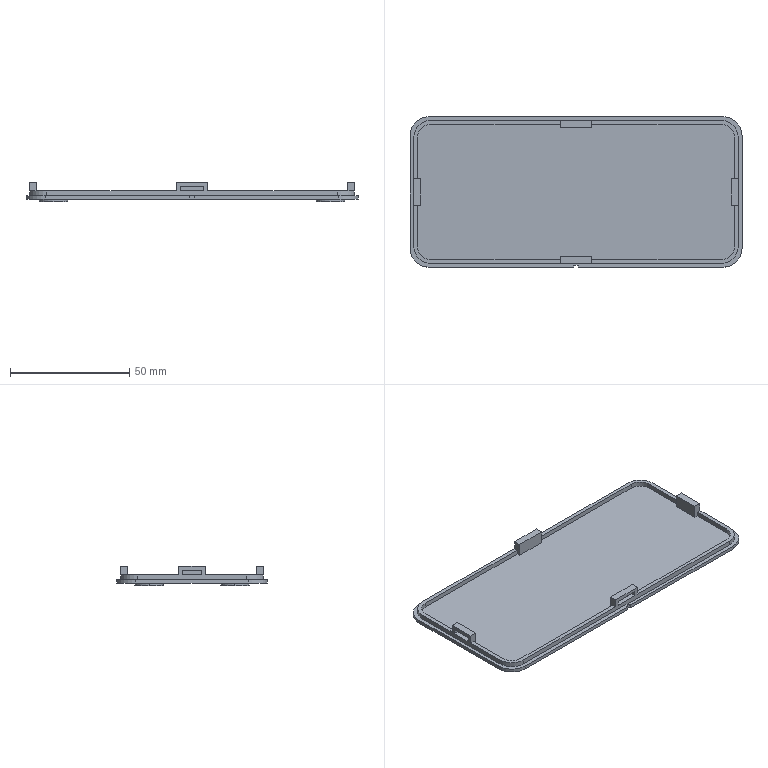Part | SolidWorks | features ICE 7, MirrorPattern 2, Extrusion 1 | 1 solid | 99 faces | box 139 x 63 x 8 mm | volume 14541 mm3 | plane 71 | cylinder 28 | commonest cylinder face diameters 10.2 x8 12 x8 10.8 x4 14 x4 16 x4